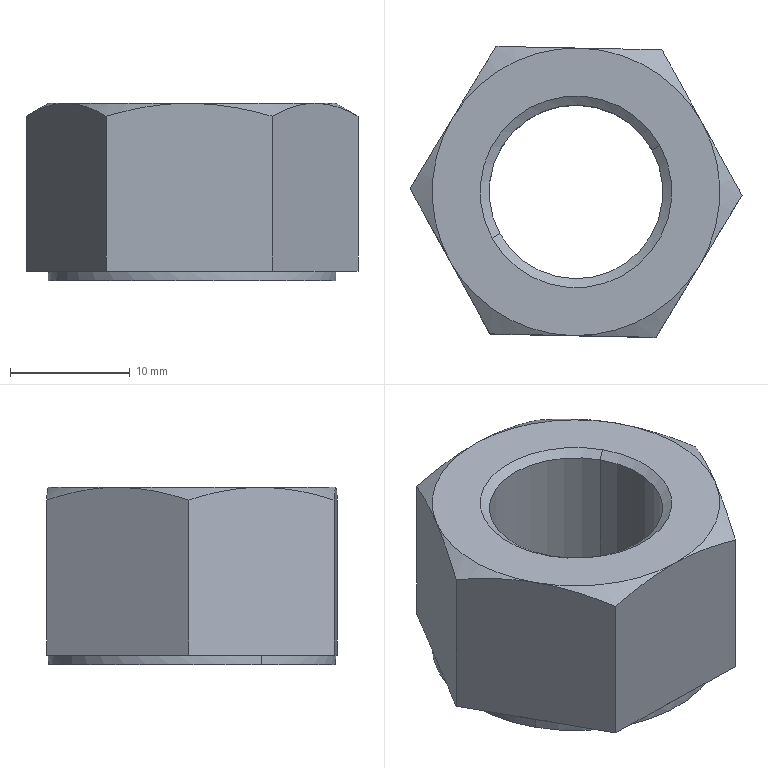Part | STEP file | Input 91 | 1 solid | 30 faces | box 27.707 x 24.281 x 14.8 mm | volume 4867 mm3 | plane 14 | cone 10 | cylinder 6 | commonest cylinder face diameters 14.5 x2 16 x2 24 x2